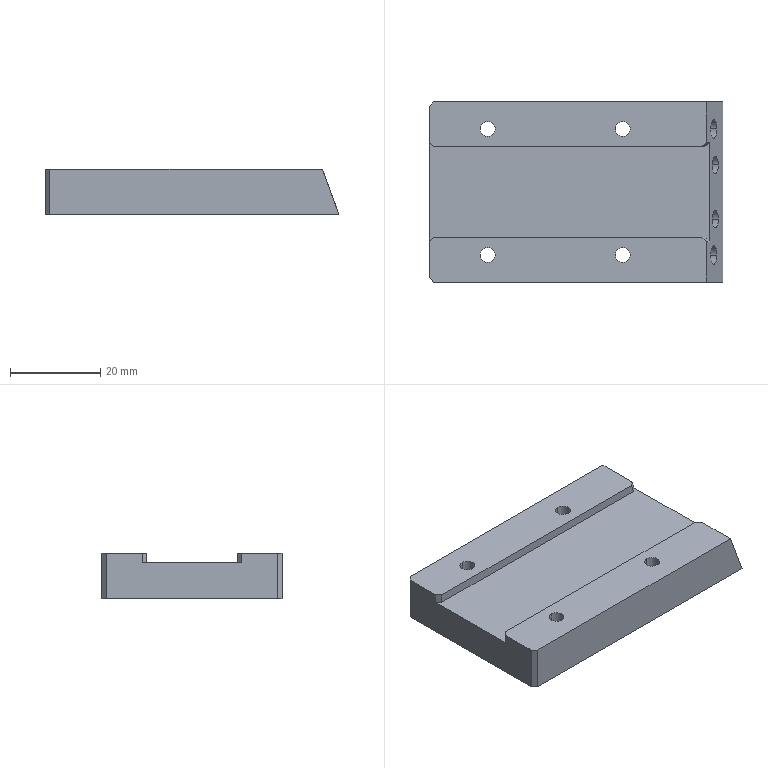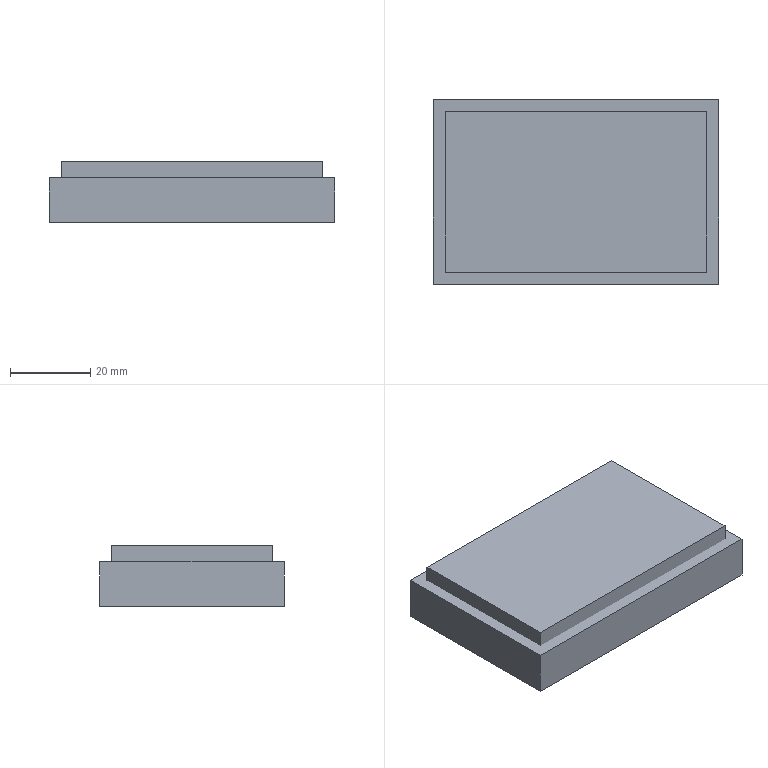CAM job | NX | 3-axis milling, drilling | part box 65.2 x 40 x 10 mm | stock box 71.2 x 46 x 15 mm
Tools:
number,name,description,diameter,corner_radius,flute_length,length,flutes
3,D50R0.8,Milling Tool-5 Parameters,50.0,0.8,50.0,75.0,2
4,D10,Milling Tool-5 Parameters,10.0,0.0,50.0,75.0,2
16,D6JING,Milling Tool-5 Parameters,6.0,0.0,50.0,75.0,2
1,D6A45,Milling Tool-5 Parameters,6.0,0.0,3.0,3.0,2
20,ZXZ,Milling Tool-5 Parameters,6.0,0.0,50.0,75.0,2
8,D6R0.5,Milling Tool-5 Parameters,6.0,0.5,50.0,75.0,2
13,3.3ZT,Drilling Tool,3.3,0.0,35.0,50.0,2
11,D2.9XYD,Thread Mill,2.9,0.0,0.7,50.0,2
12,4.2ZT,Drilling Tool,4.2,0.0,35.0,50.0,2
9,3.8ZT,Drilling Tool,3.8,0.0,35.0,50.0,2
10,4.0JD,Milling Tool-5 Parameters,4.0,0.0,30.0,30.0,4
5,D3.9XYD,Thread Mill,3.9,0.0,0.8,50.0,2
Operations:
program,operation,operation_type,tool,method,geometry_group,spindle_rpm,surface_speed,feed_per_tooth,feed_cut,feed_plunge,cut_length_mm,path_length_mm,cut_time_min,machine_time_min
1,FLOOR_WALL_COPY,VolumeBased25DMillingOperation,D50R0.8,METHOD,A,1500.0,296.0,0.3333,1000.0,100.0,133.2,187.2,0.1332,0.1386
1,ADAPTIVE_MILLING_COPY,CavityMilling,D10,METHOD,A,4000.0,125.0,0.275,2200.0,1000.0,19046.429,20593.595,8.667,8.822
1,ZLEVEL_PROFILE_1_COPY,ZLevelMilling,D6JING,METHOD,A,6500.0,122.0,0.0769,1000.0,100.0,231.953,309.953,0.232,0.2398
1,FLOOR_WALL,VolumeBased25DMillingOperation,D6JING,METHOD,A,6500.0,122.0,0.0962,1250.0,100.0,577.706,786.951,0.4622,0.4831
1,ZLEVEL_PROFILE_COPY_COPY_COPY_COPY,ZLevelMilling,D6R0.5,METHOD,A,6500.0,122.0,0.1923,2500.0,1000.0,4669.601,4932.72,1.872,1.899
1,DRILLING_COPY_1,Operation,ZXZ,METHOD,A,5000.0,94.0,0.025,250.0,0.0,16.0,187.47,0.064,0.0811
1,DRILLING_COPY_1_COPY,Operation,3.3ZT,METHOD,A,2000.0,21.0,0.0375,150.0,0.0,57.966,271.401,0.3864,0.4078
1,刀补11,ThreadMilling,D2.9XYD,METHOD,A,4000.0,36.0,0.125,1000.0,100.0,675.927,1873.927,0.6759,0.7957
1,刀补16,VolumeBased25DMillingOperation,D6JING,METHOD,A,9500.0,179.0,0.0658,1250.0,100.0,149.827,292.997,0.1199,0.1342
1,11_COPY_COPY_COPY_COPY,ZLevelMilling,D6A45,METHOD,A,7500.0,141.0,0.0667,1000.0,100.0,336.382,826.409,0.3364,0.3854
1,11_COPY_COPY_COPY_COPY_COPY,ZLevelMilling,D6A45,METHOD,A,7500.0,141.0,0.0667,1000.0,100.0,23.312,83.312,0.0233,0.0293
1,DRILLING,HoleDrilling,ZXZ,METHOD,A,3500.0,65.0,0.0357,250.0,0.0,32.0,188.626,0.064,0.0797
1,DRILLING_COPY_2,HoleDrilling,3.8ZT,METHOD,A,2000.0,23.0,0.0375,150.0,0.0,120.567,191.399,0.1219,0.129
1,DRILLING_COPY_2_COPY,HoleDrilling,4.0JD,METHOD,A,1000.0,12.0,0.0125,50.0,0.0,32.0,103.258,0.32,0.3271
1,DRILLING_COPY,HoleDrilling,4.2ZT,METHOD,A,2000.0,26.0,0.0375,150.0,0.0,233.047,322.187,0.1768,0.1857
1,刀补5,ThreadMilling,D3.9XYD,METHOD,A,4000.0,36.0,0.125,1000.0,100.0,290.794,721.165,0.2908,0.3338
2,FLOOR_WALL_COPY_COPY,VolumeBased25DMillingOperation,D50R0.8,METHOD,B,1000.0,157.0,0.75,1500.0,100.0,2162.4,4936.902,1.442,1.719
2,FLOOR_WALL_COPY_COPY_1,VolumeBased25DMillingOperation,D50R0.8,METHOD,B,1500.0,296.0,0.3333,1000.0,100.0,127.2,181.2,0.1272,0.1326
2,11_COPY_COPY_COPY_COPY_COPY_1,ZLevelMilling,D6A45,METHOD,B,7500.0,141.0,0.0667,1000.0,100.0,272.24,715.472,0.2722,0.3166